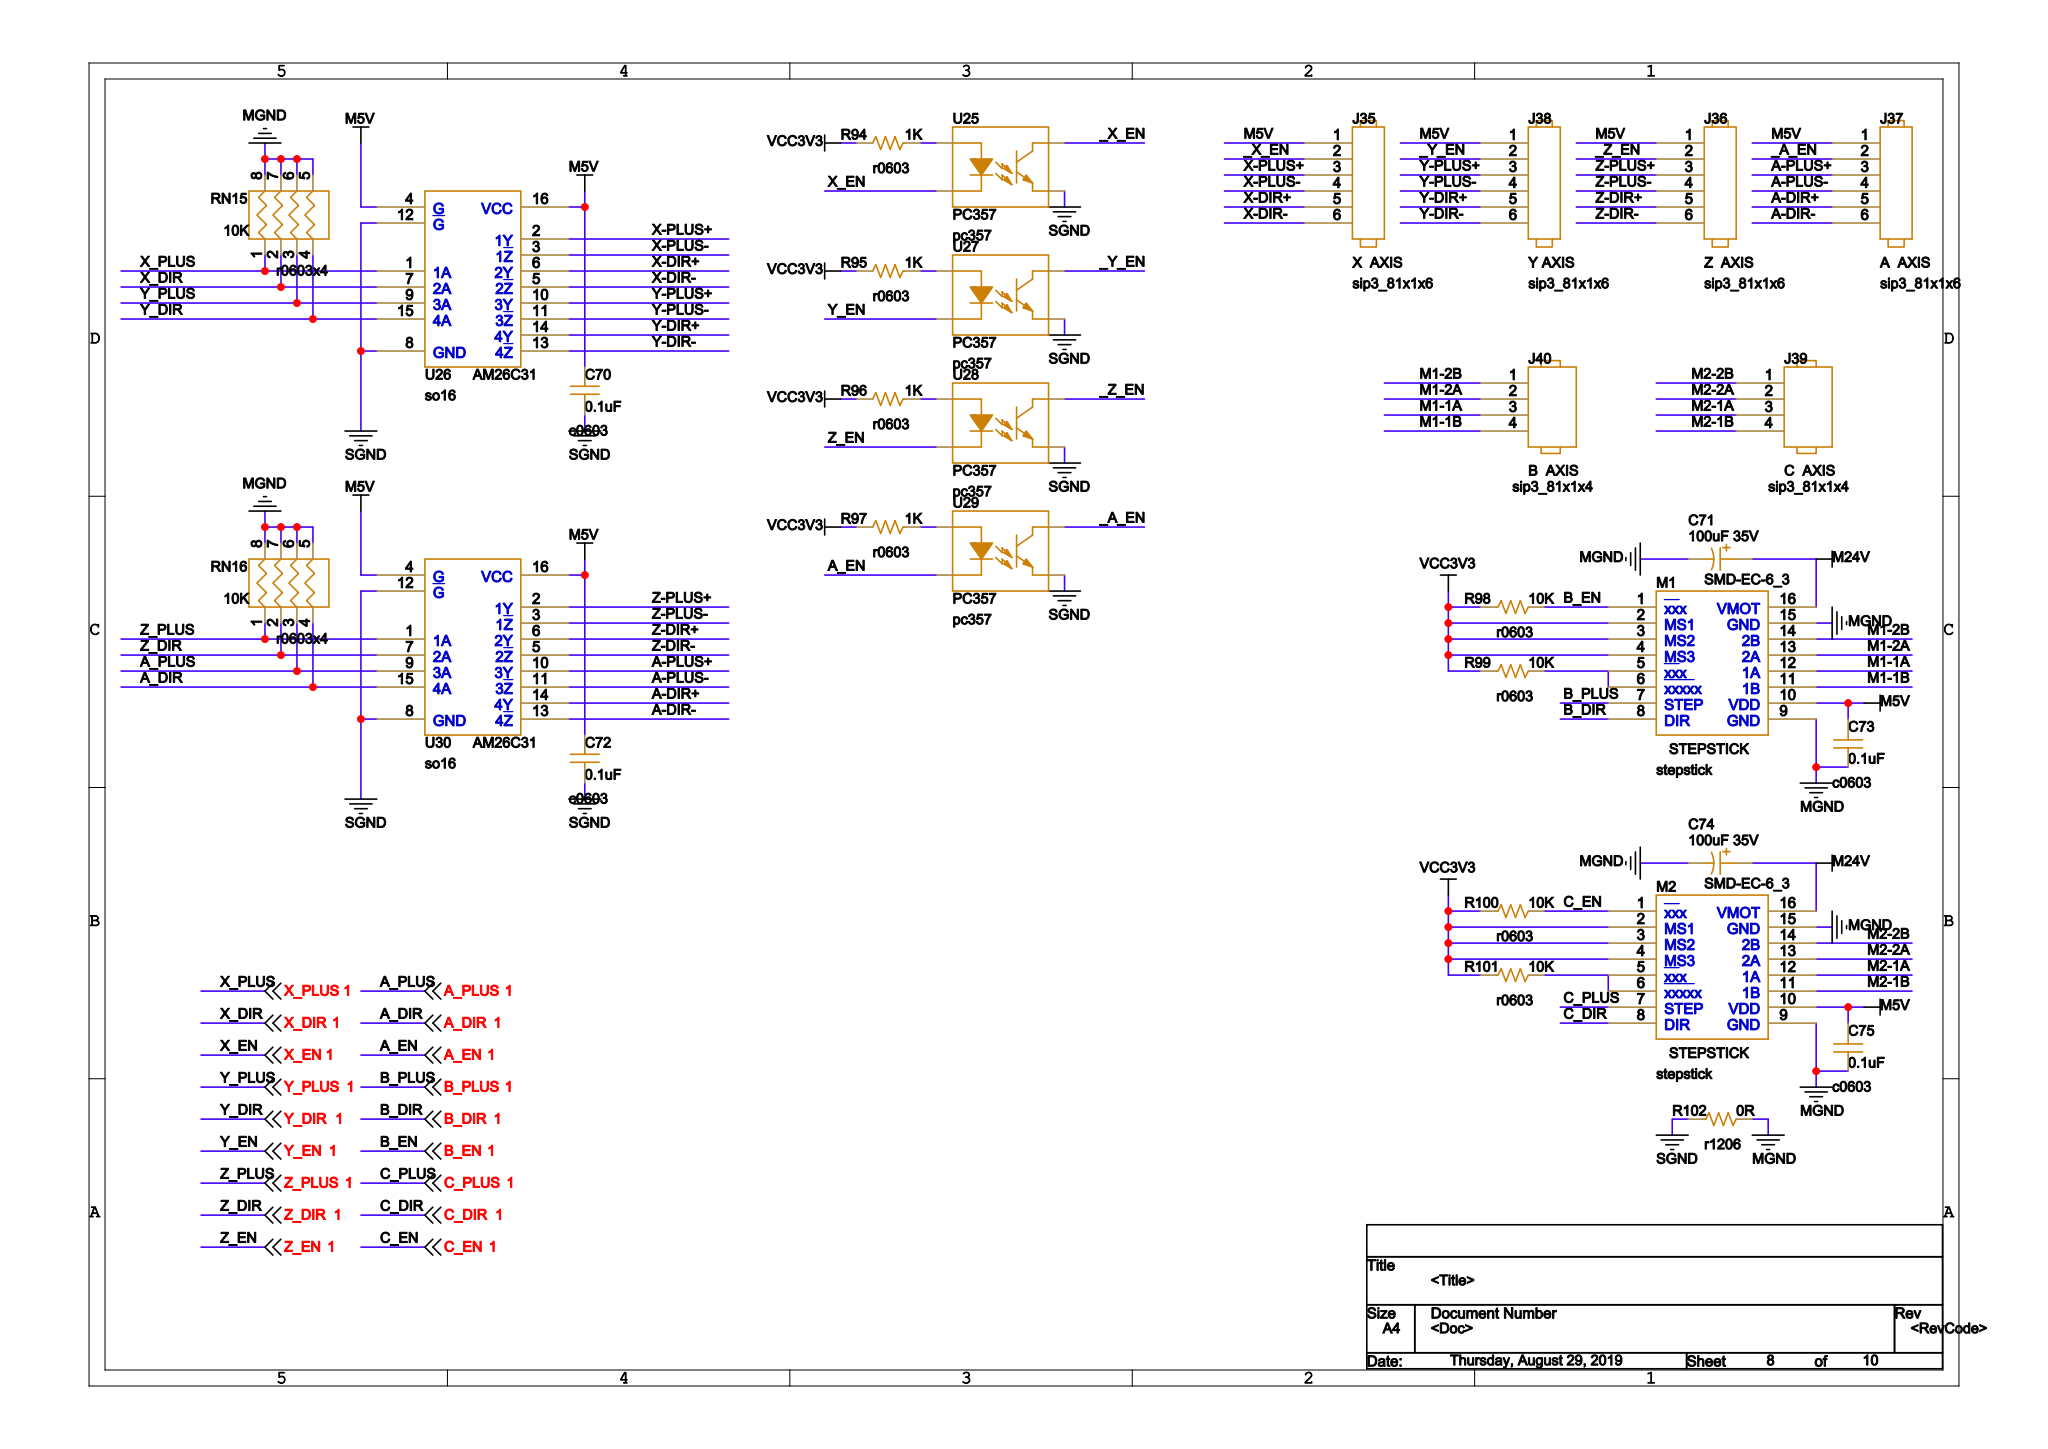Circuit board | Cadence Allegro | 380 parts | 375 nets | one sheet of the schematic
Parts on this sheet (reference | value | footprint):
C70 | 0.1uF | C0603
C71 | 100uF 35V | SMD-EC-6_3
C72 | 0.1uF | C0603
C73 | 0.1uF | C0603
C74 | 100uF 35V | SMD-EC-6_3
C75 | 0.1uF | C0603
J35 | X  AXIS | SIP3_81X1X6
J36 | Z  AXIS | SIP3_81X1X6
J37 | A  AXIS | SIP3_81X1X6
J38 | Y AXIS | SIP3_81X1X6
J39 | C  AXIS | SIP3_81X1X4
J40 | B  AXIS | SIP3_81X1X4
M1 | STEPSTICK | STEPSTICK
M2 | STEPSTICK | STEPSTICK
R94 | 1K | R0603
R95 | 1K | R0603
R96 | 1K | R0603
R97 | 1K | R0603
R98 | 10K | R0603
R99 | 10K | R0603
R100 | 10K | R0603
R101 | 10K | R0603
R102 | 0R | R1206
RN15 | 10K | R0603X4
RN16 | 10K | R0603X4
U25 | PC357 | PC357
U26 | AM26C31 | SO16
U27 | PC357 | PC357
U28 | PC357 | PC357
U29 | PC357 | PC357
U30 | AM26C31 | SO16
Nets of these parts (net: part-pin ...):
M24V: C71-1 C74-1 M1-16 M2-16
VCC3V3: M1-2 M1-3 M1-4 M2-2 M2-3 M2-4 R94-2 R95-2 R96-2 R97-2 R98-1 R99-1 R100-1 R101-1
SGND: C70-2 C72-2 R102-1 U25-3 U26-8 U26-12 U27-3 U28-3 U29-3 U30-8 U30-12
MGND: C71-2 C73-1 C74-2 C75-1 M1-9 M1-15 M2-9 M2-15 R102-2 RN15-5 RN15-6 RN15-7 RN15-8 RN16-5 RN16-6 RN16-7 RN16-8
M1-2B: J40-1 M1-14
M1-2A: J40-2 M1-13
M1-1A: J40-3 M1-12
M1-1B: J40-4 M1-11
M2-2B: J39-1 M2-14
M2-2A: J39-2 M2-13
M2-1A: J39-3 M2-12
M2-1B: J39-4 M2-11
M5V: C70-1 C72-1 C73-2 C75-2 J35-1 J36-1 J37-1 J38-1 M1-10 M2-10 U26-4 U26-16 U30-4 U30-16
_X_EN: J35-2 U25-4
X-PLUS+: J35-3 U26-2
X-PLUS-: J35-4 U26-3
X-DIR+: J35-5 U26-6
X-DIR-: J35-6 U26-5
_Z_EN: J36-2 U28-4
Z-PLUS+: J36-3 U30-2
Z-PLUS-: J36-4 U30-3
Z-DIR+: J36-5 U30-6
Z-DIR-: J36-6 U30-5
_A_EN: J37-2 U29-4
A-PLUS+: J37-3 U30-10
A-PLUS-: J37-4 U30-11
A-DIR+: J37-5 U30-14
A-DIR-: J37-6 U30-13
_Y_EN: J38-2 U27-4
Y-PLUS+: J38-3 U26-10
Y-PLUS-: J38-4 U26-11
Y-DIR+: J38-5 U26-14
Y-DIR-: J38-6 U26-13
B_DIR: M1-8
B_PLUS: M1-7
B_EN: M1-1 R98-2
N1646719: M1-5 M1-6 R99-2
C_DIR: M2-8
C_PLUS: M2-7
C_EN: M2-1 R100-2
N1647903: M2-5 M2-6 R101-2
N1604342: R94-1 U25-1
N1606045: R95-1 U27-1
N1606237: R96-1 U28-1
N1606419: R97-1 U29-1
Z_PLUS: RN16-1 U30-1
Z_DIR: RN16-2 U30-7
A_PLUS: RN16-3 U30-9
A_DIR: RN16-4 U30-15
X_PLUS: RN15-1 U26-1
X_DIR: RN15-2 U26-7
Y_PLUS: RN15-3 U26-9
Y_DIR: RN15-4 U26-15
Y_EN: U27-2
X_EN: U25-2
A_EN: U29-2
Z_EN: U28-2